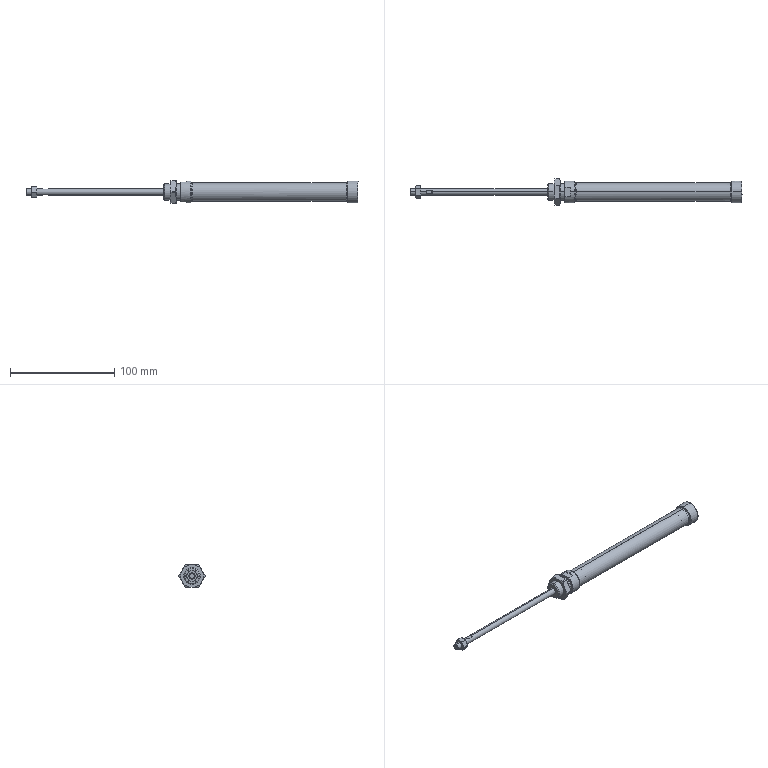Part | SolidWorks | 4 solids | 124 faces | box 318 x 25 x 22 mm | volume 45425 mm3 | plane 41 | cone 39 | cylinder 36 | spline 8 | commonest cylinder face diameters 17.4 x6 25 x6 4.134 x4 6 x4 16 x4 21 x4